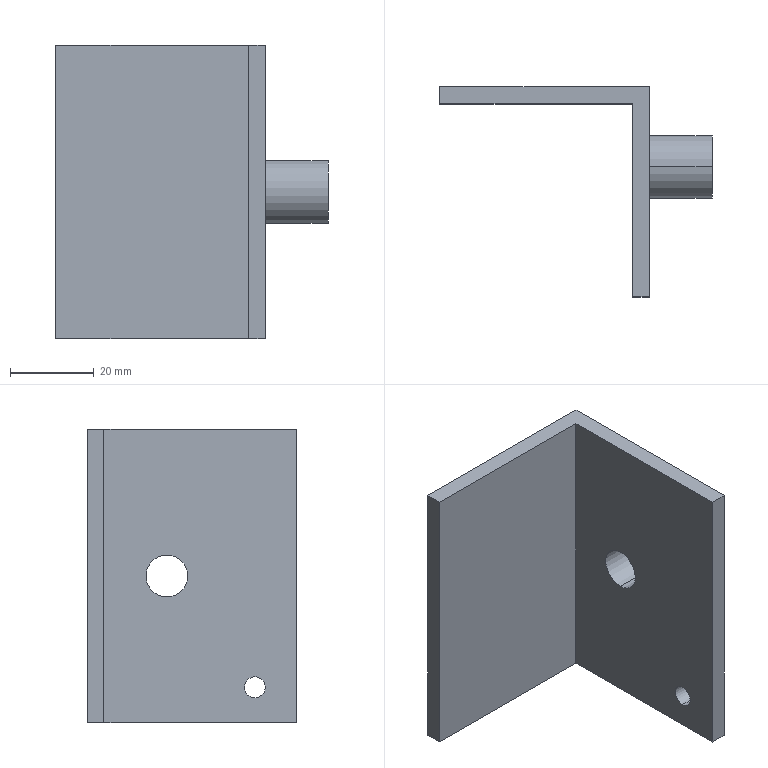Part | STEP file | 1 solid | 15 faces | box 65 x 50 x 70 mm | volume 27960 mm3 | plane 9 | cylinder 6 | commonest cylinder face diameters 5 x2 10 x2 15 x2
STEP:
#1=CARTESIAN_POINT('',(0.,0.,0.));
#2=DIRECTION('',(0.,0.,1.));
#3=DIRECTION('',(1.,0.,0.));
#4=AXIS2_PLACEMENT_3D('',#1,#2,#3);
#5=CARTESIAN_POINT('',(34.103,0.4017,42.5));
#6=VERTEX_POINT('',#5);
#7=CARTESIAN_POINT('',(34.103,0.4017,27.5));
#8=VERTEX_POINT('',#7);
#9=CARTESIAN_POINT('',(34.103,0.4017,35.));
#10=DIRECTION('',(-1.,0.,0.));
#11=DIRECTION('',(0.,0.,-1.));
#12=AXIS2_PLACEMENT_3D('',#9,#10,#11);
#13=CIRCLE('',#12,7.5);
#14=CARTESIAN_POINT('',(34.103,0.4017,35.));
#15=DIRECTION('',(1.,0.,0.));
#16=DIRECTION('',(0.,0.,-1.));
#17=AXIS2_PLACEMENT_3D('',#14,#15,#16);
#18=CYLINDRICAL_SURFACE('',#17,7.5);
#19=CARTESIAN_POINT('',(6.283,0.));
#20=DIRECTION('',(-1.,0.));
#21=VECTOR('',#20,1.);
#22=LINE('',#19,#21);
#23=(GEOMETRIC_REPRESENTATION_CONTEXT(2)PARAMETRIC_REPRESENTATION_CONTEXT()REPRESENTATION_CONTEXT('',''));
#24=DEFINITIONAL_REPRESENTATION('',(#22),#23);
#25=PCURVE('',#18,#24);
#26=CARTESIAN_POINT('',(34.103,-30.598,0.));
#27=DIRECTION('',(1.,0.,0.));
#28=DIRECTION('',(0.,0.,-1.));
#29=AXIS2_PLACEMENT_3D('',#26,#27,#28);
#30=PLANE('',#29);
#31=CARTESIAN_POINT('',(-27.5,31.));
#32=CARTESIAN_POINT('',(-27.5,18.01));
#33=CARTESIAN_POINT('',(-38.75,24.505));
#34=CARTESIAN_POINT('',(-50.,31.));
#35=CARTESIAN_POINT('',(-38.75,37.495));
#36=CARTESIAN_POINT('',(-27.5,43.99));
#37=CARTESIAN_POINT('',(-27.5,31.));
#38=(BOUNDED_CURVE()B_SPLINE_CURVE(2,(#31,#32,#33,#34,#35,#36,#37),.UNSPECIFIED.,.T.,.F.)B_SPLINE_CURVE_WITH_KNOTS((1,2,2,2,2,1),(-2.094,0.,2.094,4.189,6.283,8.378),.UNSPECIFIED.)CURVE()GEOMETRIC_REPRESENTATION_ITEM()RATIONAL_B_SPLINE_CURVE((1.,0.5,1.,0.5,1.,0.5,1.))REPRESENTATION_ITEM(''));
#39=(GEOMETRIC_REPRESENTATION_CONTEXT(2)PARAMETRIC_REPRESENTATION_CONTEXT()REPRESENTATION_CONTEXT('',''));
#40=DEFINITIONAL_REPRESENTATION('',(#38),#39);
#41=PCURVE('',#30,#40);
#42=SURFACE_CURVE('',#13,(#25,#41),.PCURVE_S1.);
#43=EDGE_CURVE('',#6,#8,#42,.T.);
#44=ORIENTED_EDGE('',*,*,#43,.F.);
#45=CARTESIAN_POINT('',(49.103,0.4017,42.5));
#46=VERTEX_POINT('',#45);
#47=CARTESIAN_POINT('',(34.103,0.4017,42.5));
#48=DIRECTION('',(1.,0.,0.));
#49=VECTOR('',#48,1.);
#50=LINE('',#47,#49);
#51=CARTESIAN_POINT('',(3.142,0.));
#52=DIRECTION('',(0.,1.));
#53=VECTOR('',#52,1.);
#54=LINE('',#51,#53);
#55=(GEOMETRIC_REPRESENTATION_CONTEXT(2)PARAMETRIC_REPRESENTATION_CONTEXT()REPRESENTATION_CONTEXT('',''));
#56=DEFINITIONAL_REPRESENTATION('',(#54),#55);
#57=PCURVE('',#18,#56);
#58=CARTESIAN_POINT('',(34.103,0.4017,35.));
#59=DIRECTION('',(1.,0.,0.));
#60=DIRECTION('',(0.,0.,-1.));
#61=AXIS2_PLACEMENT_3D('',#58,#59,#60);
#62=CYLINDRICAL_SURFACE('',#61,7.5);
#63=CARTESIAN_POINT('',(3.142,0.));
#64=DIRECTION('',(0.,1.));
#65=VECTOR('',#64,1.);
#66=LINE('',#63,#65);
#67=(GEOMETRIC_REPRESENTATION_CONTEXT(2)PARAMETRIC_REPRESENTATION_CONTEXT()REPRESENTATION_CONTEXT('',''));
#68=DEFINITIONAL_REPRESENTATION('',(#66),#67);
#69=PCURVE('',#62,#68);
#70=SURFACE_CURVE('',#50,(#57,#69),.PCURVE_S1.);
#71=EDGE_CURVE('',#6,#46,#70,.T.);
#72=ORIENTED_EDGE('',*,*,#71,.T.);
#73=CARTESIAN_POINT('',(49.103,0.4017,27.5));
#74=VERTEX_POINT('',#73);
#75=CARTESIAN_POINT('',(49.103,0.4017,35.));
#76=DIRECTION('',(-1.,0.,0.));
#77=DIRECTION('',(0.,0.,-1.));
#78=AXIS2_PLACEMENT_3D('',#75,#76,#77);
#79=CIRCLE('',#78,7.5);
#80=CARTESIAN_POINT('',(6.283,15.));
#81=DIRECTION('',(-1.,0.));
#82=VECTOR('',#81,1.);
#83=LINE('',#80,#82);
#84=(GEOMETRIC_REPRESENTATION_CONTEXT(2)PARAMETRIC_REPRESENTATION_CONTEXT()REPRESENTATION_CONTEXT('',''));
#85=DEFINITIONAL_REPRESENTATION('',(#83),#84);
#86=PCURVE('',#18,#85);
#87=CARTESIAN_POINT('',(49.103,0.4017,35.));
#88=DIRECTION('',(1.,0.,0.));
#89=DIRECTION('',(0.,0.,-1.));
#90=AXIS2_PLACEMENT_3D('',#87,#88,#89);
#91=PLANE('',#90);
#92=CARTESIAN_POINT('',(7.5,0.));
#93=CARTESIAN_POINT('',(7.5,-12.99));
#94=CARTESIAN_POINT('',(-3.75,-6.495));
#95=CARTESIAN_POINT('',(-15.,0.));
#96=CARTESIAN_POINT('',(-3.75,6.495));
#97=CARTESIAN_POINT('',(7.5,12.99));
#98=CARTESIAN_POINT('',(7.5,0.));
#99=(BOUNDED_CURVE()B_SPLINE_CURVE(2,(#92,#93,#94,#95,#96,#97,#98),.UNSPECIFIED.,.T.,.F.)B_SPLINE_CURVE_WITH_KNOTS((1,2,2,2,2,1),(-2.094,0.,2.094,4.189,6.283,8.378),.UNSPECIFIED.)CURVE()GEOMETRIC_REPRESENTATION_ITEM()RATIONAL_B_SPLINE_CURVE((1.,0.5,1.,0.5,1.,0.5,1.))REPRESENTATION_ITEM(''));
#100=(GEOMETRIC_REPRESENTATION_CONTEXT(2)PARAMETRIC_REPRESENTATION_CONTEXT()REPRESENTATION_CONTEXT('',''));
#101=DEFINITIONAL_REPRESENTATION('',(#99),#100);
#102=PCURVE('',#91,#101);
#103=SURFACE_CURVE('',#79,(#86,#102),.PCURVE_S1.);
#104=EDGE_CURVE('',#46,#74,#103,.T.);
#105=ORIENTED_EDGE('',*,*,#104,.T.);
#106=CARTESIAN_POINT('',(34.103,0.4017,27.5));
#107=DIRECTION('',(1.,0.,0.));
#108=VECTOR('',#107,1.);
#109=LINE('',#106,#108);
#110=CARTESIAN_POINT('',(0.,0.));
#111=DIRECTION('',(0.,1.));
#112=VECTOR('',#111,1.);
#113=LINE('',#110,#112);
#114=(GEOMETRIC_REPRESENTATION_CONTEXT(2)PARAMETRIC_REPRESENTATION_CONTEXT()REPRESENTATION_CONTEXT('',''));
#115=DEFINITIONAL_REPRESENTATION('',(#113),#114);
#116=PCURVE('',#18,#115);
#117=CARTESIAN_POINT('',(6.283,0.));
#118=DIRECTION('',(0.,1.));
#119=VECTOR('',#118,1.);
#120=LINE('',#117,#119);
#121=(GEOMETRIC_REPRESENTATION_CONTEXT(2)PARAMETRIC_REPRESENTATION_CONTEXT()REPRESENTATION_CONTEXT('',''));
#122=DEFINITIONAL_REPRESENTATION('',(#120),#121);
#123=PCURVE('',#62,#122);
#124=SURFACE_CURVE('',#109,(#116,#123),.PCURVE_S1.);
#125=EDGE_CURVE('',#8,#74,#124,.T.);
#126=ORIENTED_EDGE('',*,*,#125,.F.);
#127=EDGE_LOOP('',(#44,#72,#105,#126));
#128=FACE_BOUND('',#127,.T.);
#129=ADVANCED_FACE('',(#128),#18,.T.);
#130=CARTESIAN_POINT('',(34.103,-20.598,10.952));
#131=VERTEX_POINT('',#130);
#132=CARTESIAN_POINT('',(30.103,-20.598,10.952));
#133=VERTEX_POINT('',#132);
#134=CARTESIAN_POINT('',(34.103,-20.598,10.952));
#135=DIRECTION('',(-1.,0.,0.));
#136=VECTOR('',#135,1.);
#137=LINE('',#134,#136);
#138=CARTESIAN_POINT('',(34.103,-20.598,8.452));
#139=DIRECTION('',(-1.,0.,0.));
#140=DIRECTION('',(0.,0.,1.));
#141=AXIS2_PLACEMENT_3D('',#138,#139,#140);
#142=CYLINDRICAL_SURFACE('',#141,2.5);
#143=CARTESIAN_POINT('',(6.283,0.));
#144=DIRECTION('',(0.,1.));
#145=VECTOR('',#144,1.);
#146=LINE('',#143,#145);
#147=(GEOMETRIC_REPRESENTATION_CONTEXT(2)PARAMETRIC_REPRESENTATION_CONTEXT()REPRESENTATION_CONTEXT('',''));
#148=DEFINITIONAL_REPRESENTATION('',(#146),#147);
#149=PCURVE('',#142,#148);
#150=CARTESIAN_POINT('',(34.103,-20.598,8.452));
#151=DIRECTION('',(-1.,0.,0.));
#152=DIRECTION('',(0.,0.,1.));
#153=AXIS2_PLACEMENT_3D('',#150,#151,#152);
#154=CYLINDRICAL_SURFACE('',#153,2.5);
#155=CARTESIAN_POINT('',(0.,0.));
#156=DIRECTION('',(0.,1.));
#157=VECTOR('',#156,1.);
#158=LINE('',#155,#157);
#159=(GEOMETRIC_REPRESENTATION_CONTEXT(2)PARAMETRIC_REPRESENTATION_CONTEXT()REPRESENTATION_CONTEXT('',''));
#160=DEFINITIONAL_REPRESENTATION('',(#158),#159);
#161=PCURVE('',#154,#160);
#162=SURFACE_CURVE('',#137,(#149,#161),.PCURVE_S1.);
#163=EDGE_CURVE('',#131,#133,#162,.T.);
#164=ORIENTED_EDGE('',*,*,#163,.T.);
#165=CARTESIAN_POINT('',(30.103,-20.598,5.952));
#166=VERTEX_POINT('',#165);
#167=CARTESIAN_POINT('',(30.103,-20.598,8.452));
#168=DIRECTION('',(1.,0.,0.));
#169=DIRECTION('',(0.,0.,1.));
#170=AXIS2_PLACEMENT_3D('',#167,#168,#169);
#171=CIRCLE('',#170,2.5);
#172=CARTESIAN_POINT('',(6.283,4.));
#173=DIRECTION('',(-1.,0.));
#174=VECTOR('',#173,1.);
#175=LINE('',#172,#174);
#176=(GEOMETRIC_REPRESENTATION_CONTEXT(2)PARAMETRIC_REPRESENTATION_CONTEXT()REPRESENTATION_CONTEXT('',''));
#177=DEFINITIONAL_REPRESENTATION('',(#175),#176);
#178=PCURVE('',#142,#177);
#179=CARTESIAN_POINT('',(30.103,15.402,0.));
#180=DIRECTION('',(-1.,0.,0.));
#181=DIRECTION('',(0.,-1.,0.));
#182=AXIS2_PLACEMENT_3D('',#179,#180,#181);
#183=PLANE('',#182);
#184=CARTESIAN_POINT('',(36.,10.952));
#185=CARTESIAN_POINT('',(40.33,10.952));
#186=CARTESIAN_POINT('',(38.165,7.202));
#187=CARTESIAN_POINT('',(36.,3.452));
#188=CARTESIAN_POINT('',(33.835,7.202));
#189=CARTESIAN_POINT('',(31.67,10.952));
#190=CARTESIAN_POINT('',(36.,10.952));
#191=(BOUNDED_CURVE()B_SPLINE_CURVE(2,(#184,#185,#186,#187,#188,#189,#190),.UNSPECIFIED.,.T.,.F.)B_SPLINE_CURVE_WITH_KNOTS((1,2,2,2,2,1),(-2.094,0.,2.094,4.189,6.283,8.378),.UNSPECIFIED.)CURVE()GEOMETRIC_REPRESENTATION_ITEM()RATIONAL_B_SPLINE_CURVE((1.,0.5,1.,0.5,1.,0.5,1.))REPRESENTATION_ITEM(''));
#192=(GEOMETRIC_REPRESENTATION_CONTEXT(2)PARAMETRIC_REPRESENTATION_CONTEXT()REPRESENTATION_CONTEXT('',''));
#193=DEFINITIONAL_REPRESENTATION('',(#191),#192);
#194=PCURVE('',#183,#193);
#195=SURFACE_CURVE('',#171,(#178,#194),.PCURVE_S1.);
#196=EDGE_CURVE('',#133,#166,#195,.T.);
#197=ORIENTED_EDGE('',*,*,#196,.T.);
#198=CARTESIAN_POINT('',(34.103,-20.598,5.952));
#199=VERTEX_POINT('',#198);
#200=CARTESIAN_POINT('',(34.103,-20.598,5.952));
#201=DIRECTION('',(-1.,0.,0.));
#202=VECTOR('',#201,1.);
#203=LINE('',#200,#202);
#204=CARTESIAN_POINT('',(3.142,0.));
#205=DIRECTION('',(0.,1.));
#206=VECTOR('',#205,1.);
#207=LINE('',#204,#206);
#208=(GEOMETRIC_REPRESENTATION_CONTEXT(2)PARAMETRIC_REPRESENTATION_CONTEXT()REPRESENTATION_CONTEXT('',''));
#209=DEFINITIONAL_REPRESENTATION('',(#207),#208);
#210=PCURVE('',#142,#209);
#211=CARTESIAN_POINT('',(3.142,0.));
#212=DIRECTION('',(0.,1.));
#213=VECTOR('',#212,1.);
#214=LINE('',#211,#213);
#215=(GEOMETRIC_REPRESENTATION_CONTEXT(2)PARAMETRIC_REPRESENTATION_CONTEXT()REPRESENTATION_CONTEXT('',''));
#216=DEFINITIONAL_REPRESENTATION('',(#214),#215);
#217=PCURVE('',#154,#216);
#218=SURFACE_CURVE('',#203,(#210,#217),.PCURVE_S1.);
#219=EDGE_CURVE('',#199,#166,#218,.T.);
#220=ORIENTED_EDGE('',*,*,#219,.F.);
#221=CARTESIAN_POINT('',(34.103,-20.598,8.452));
#222=DIRECTION('',(-1.,0.,0.));
#223=DIRECTION('',(0.,0.,1.));
#224=AXIS2_PLACEMENT_3D('',#221,#222,#223);
#225=CIRCLE('',#224,2.5);
#226=CARTESIAN_POINT('',(0.,0.));
#227=DIRECTION('',(1.,0.));
#228=VECTOR('',#227,1.);
#229=LINE('',#226,#228);
#230=(GEOMETRIC_REPRESENTATION_CONTEXT(2)PARAMETRIC_REPRESENTATION_CONTEXT()REPRESENTATION_CONTEXT('',''));
#231=DEFINITIONAL_REPRESENTATION('',(#229),#230);
#232=PCURVE('',#142,#231);
#233=CARTESIAN_POINT('',(-10.952,10.));
#234=CARTESIAN_POINT('',(-10.952,14.33));
#235=CARTESIAN_POINT('',(-7.202,12.165));
#236=CARTESIAN_POINT('',(-3.452,10.));
#237=CARTESIAN_POINT('',(-7.202,7.835));
#238=CARTESIAN_POINT('',(-10.952,5.67));
#239=CARTESIAN_POINT('',(-10.952,10.));
#240=(BOUNDED_CURVE()B_SPLINE_CURVE(2,(#233,#234,#235,#236,#237,#238,#239),.UNSPECIFIED.,.T.,.F.)B_SPLINE_CURVE_WITH_KNOTS((1,2,2,2,2,1),(-2.094,0.,2.094,4.189,6.283,8.378),.UNSPECIFIED.)CURVE()GEOMETRIC_REPRESENTATION_ITEM()RATIONAL_B_SPLINE_CURVE((1.,0.5,1.,0.5,1.,0.5,1.))REPRESENTATION_ITEM(''));
#241=(GEOMETRIC_REPRESENTATION_CONTEXT(2)PARAMETRIC_REPRESENTATION_CONTEXT()REPRESENTATION_CONTEXT('',''));
#242=DEFINITIONAL_REPRESENTATION('',(#240),#241);
#243=PCURVE('',#30,#242);
#244=SURFACE_CURVE('',#225,(#232,#243),.PCURVE_S1.);
#245=EDGE_CURVE('',#199,#131,#244,.T.);
#246=ORIENTED_EDGE('',*,*,#245,.T.);
#247=EDGE_LOOP('',(#164,#197,#220,#246));
#248=FACE_BOUND('',#247,.F.);
#249=ADVANCED_FACE('',(#248),#142,.F.);
#250=CARTESIAN_POINT('',(30.103,0.4017,30.));
#251=VERTEX_POINT('',#250);
#252=CARTESIAN_POINT('',(49.103,0.4017,30.));
#253=VERTEX_POINT('',#252);
#254=CARTESIAN_POINT('',(34.103,0.4017,30.));
#255=DIRECTION('',(1.,0.,0.));
#256=VECTOR('',#255,1.);
#257=LINE('',#254,#256);
#258=CARTESIAN_POINT('',(34.103,0.4017,35.));
#259=DIRECTION('',(1.,0.,0.));
#260=DIRECTION('',(0.,0.,-1.));
#261=AXIS2_PLACEMENT_3D('',#258,#259,#260);
#262=CYLINDRICAL_SURFACE('',#261,5.);
#263=CARTESIAN_POINT('',(6.283,0.));
#264=DIRECTION('',(0.,1.));
#265=VECTOR('',#264,1.);
#266=LINE('',#263,#265);
#267=(GEOMETRIC_REPRESENTATION_CONTEXT(2)PARAMETRIC_REPRESENTATION_CONTEXT()REPRESENTATION_CONTEXT('',''));
#268=DEFINITIONAL_REPRESENTATION('',(#266),#267);
#269=PCURVE('',#262,#268);
#270=CARTESIAN_POINT('',(34.103,0.4017,35.));
#271=DIRECTION('',(1.,0.,0.));
#272=DIRECTION('',(0.,0.,-1.));
#273=AXIS2_PLACEMENT_3D('',#270,#271,#272);
#274=CYLINDRICAL_SURFACE('',#273,5.);
#275=CARTESIAN_POINT('',(0.,0.));
#276=DIRECTION('',(0.,1.));
#277=VECTOR('',#276,1.);
#278=LINE('',#275,#277);
#279=(GEOMETRIC_REPRESENTATION_CONTEXT(2)PARAMETRIC_REPRESENTATION_CONTEXT()REPRESENTATION_CONTEXT('',''));
#280=DEFINITIONAL_REPRESENTATION('',(#278),#279);
#281=PCURVE('',#274,#280);
#282=SURFACE_CURVE('',#257,(#269,#281),.PCURVE_S1.);
#283=EDGE_CURVE('',#251,#253,#282,.T.);
#284=ORIENTED_EDGE('',*,*,#283,.T.);
#285=CARTESIAN_POINT('',(49.103,0.4017,40.));
#286=VERTEX_POINT('',#285);
#287=CARTESIAN_POINT('',(49.103,0.4017,35.));
#288=DIRECTION('',(-1.,0.,0.));
#289=DIRECTION('',(0.,0.,-1.));
#290=AXIS2_PLACEMENT_3D('',#287,#288,#289);
#291=CIRCLE('',#290,5.);
#292=CARTESIAN_POINT('',(6.283,15.));
#293=DIRECTION('',(-1.,0.));
#294=VECTOR('',#293,1.);
#295=LINE('',#292,#294);
#296=(GEOMETRIC_REPRESENTATION_CONTEXT(2)PARAMETRIC_REPRESENTATION_CONTEXT()REPRESENTATION_CONTEXT('',''));
#297=DEFINITIONAL_REPRESENTATION('',(#295),#296);
#298=PCURVE('',#262,#297);
#299=CARTESIAN_POINT('',(5.,0.));
#300=CARTESIAN_POINT('',(5.,-8.66));
#301=CARTESIAN_POINT('',(-2.5,-4.33));
#302=CARTESIAN_POINT('',(-10.,0.));
#303=CARTESIAN_POINT('',(-2.5,4.33));
#304=CARTESIAN_POINT('',(5.,8.66));
#305=CARTESIAN_POINT('',(5.,0.));
#306=(BOUNDED_CURVE()B_SPLINE_CURVE(2,(#299,#300,#301,#302,#303,#304,#305),.UNSPECIFIED.,.T.,.F.)B_SPLINE_CURVE_WITH_KNOTS((1,2,2,2,2,1),(-2.094,0.,2.094,4.189,6.283,8.378),.UNSPECIFIED.)CURVE()GEOMETRIC_REPRESENTATION_ITEM()RATIONAL_B_SPLINE_CURVE((1.,0.5,1.,0.5,1.,0.5,1.))REPRESENTATION_ITEM(''));
#307=(GEOMETRIC_REPRESENTATION_CONTEXT(2)PARAMETRIC_REPRESENTATION_CONTEXT()REPRESENTATION_CONTEXT('',''));
#308=DEFINITIONAL_REPRESENTATION('',(#306),#307);
#309=PCURVE('',#91,#308);
#310=SURFACE_CURVE('',#291,(#298,#309),.PCURVE_S1.);
#311=EDGE_CURVE('',#253,#286,#310,.T.);
#312=ORIENTED_EDGE('',*,*,#311,.T.);
#313=CARTESIAN_POINT('',(30.103,0.4017,40.));
#314=VERTEX_POINT('',#313);
#315=CARTESIAN_POINT('',(34.103,0.4017,40.));
#316=DIRECTION('',(1.,0.,0.));
#317=VECTOR('',#316,1.);
#318=LINE('',#315,#317);
#319=CARTESIAN_POINT('',(3.142,0.));
#320=DIRECTION('',(0.,1.));
#321=VECTOR('',#320,1.);
#322=LINE('',#319,#321);
#323=(GEOMETRIC_REPRESENTATION_CONTEXT(2)PARAMETRIC_REPRESENTATION_CONTEXT()REPRESENTATION_CONTEXT('',''));
#324=DEFINITIONAL_REPRESENTATION('',(#322),#323);
#325=PCURVE('',#262,#324);
#326=CARTESIAN_POINT('',(3.142,0.));
#327=DIRECTION('',(0.,1.));
#328=VECTOR('',#327,1.);
#329=LINE('',#326,#328);
#330=(GEOMETRIC_REPRESENTATION_CONTEXT(2)PARAMETRIC_REPRESENTATION_CONTEXT()REPRESENTATION_CONTEXT('',''));
#331=DEFINITIONAL_REPRESENTATION('',(#329),#330);
#332=PCURVE('',#274,#331);
#333=SURFACE_CURVE('',#318,(#325,#332),.PCURVE_S1.);
#334=EDGE_CURVE('',#314,#286,#333,.T.);
#335=ORIENTED_EDGE('',*,*,#334,.F.);
#336=CARTESIAN_POINT('',(30.103,0.4017,35.));
#337=DIRECTION('',(1.,0.,0.));
#338=DIRECTION('',(0.,0.,-1.));
#339=AXIS2_PLACEMENT_3D('',#336,#337,#338);
#340=CIRCLE('',#339,5.);
#341=CARTESIAN_POINT('',(0.,-4.));
#342=DIRECTION('',(1.,0.));
#343=VECTOR('',#342,1.);
#344=LINE('',#341,#343);
#345=(GEOMETRIC_REPRESENTATION_CONTEXT(2)PARAMETRIC_REPRESENTATION_CONTEXT()REPRESENTATION_CONTEXT('',''));
#346=DEFINITIONAL_REPRESENTATION('',(#344),#345);
#347=PCURVE('',#262,#346);
#348=CARTESIAN_POINT('',(15.,30.));
#349=CARTESIAN_POINT('',(6.34,30.));
#350=CARTESIAN_POINT('',(10.67,37.5));
#351=CARTESIAN_POINT('',(15.,45.));
#352=CARTESIAN_POINT('',(19.33,37.5));
#353=CARTESIAN_POINT('',(23.66,30.));
#354=CARTESIAN_POINT('',(15.,30.));
#355=(BOUNDED_CURVE()B_SPLINE_CURVE(2,(#348,#349,#350,#351,#352,#353,#354),.UNSPECIFIED.,.T.,.F.)B_SPLINE_CURVE_WITH_KNOTS((1,2,2,2,2,1),(-2.094,0.,2.094,4.189,6.283,8.378),.UNSPECIFIED.)CURVE()GEOMETRIC_REPRESENTATION_ITEM()RATIONAL_B_SPLINE_CURVE((1.,0.5,1.,0.5,1.,0.5,1.))REPRESENTATION_ITEM(''));
#356=(GEOMETRIC_REPRESENTATION_CONTEXT(2)PARAMETRIC_REPRESENTATION_CONTEXT()REPRESENTATION_CONTEXT('',''));
#357=DEFINITIONAL_REPRESENTATION('',(#355),#356);
#358=PCURVE('',#183,#357);
#359=SURFACE_CURVE('',#340,(#347,#358),.PCURVE_S1.);
#360=EDGE_CURVE('',#314,#251,#359,.T.);
#361=ORIENTED_EDGE('',*,*,#360,.T.);
#362=EDGE_LOOP('',(#284,#312,#335,#361));
#363=FACE_BOUND('',#362,.F.);
#364=ADVANCED_FACE('',(#363),#262,.F.);
#365=CARTESIAN_POINT('',(-15.897,19.402,70.));
#366=VERTEX_POINT('',#365);
#367=CARTESIAN_POINT('',(34.103,19.402,70.));
#368=VERTEX_POINT('',#367);
#369=CARTESIAN_POINT('',(34.103,19.402,70.));
#370=DIRECTION('',(1.,0.,0.));
#371=VECTOR('',#370,1.);
#372=LINE('',#369,#371);
#373=CARTESIAN_POINT('',(34.103,19.402,0.));
#374=DIRECTION('',(0.,1.,0.));
#375=DIRECTION('',(0.,0.,1.));
#376=AXIS2_PLACEMENT_3D('',#373,#374,#375);
#377=PLANE('',#376);
#378=CARTESIAN_POINT('',(70.,0.));
#379=DIRECTION('',(0.,1.));
#380=VECTOR('',#379,1.);
#381=LINE('',#378,#380);
#382=(GEOMETRIC_REPRESENTATION_CONTEXT(2)PARAMETRIC_REPRESENTATION_CONTEXT()REPRESENTATION_CONTEXT('',''));
#383=DEFINITIONAL_REPRESENTATION('',(#381),#382);
#384=PCURVE('',#377,#383);
#385=CARTESIAN_POINT('',(19.683,4.982,70.));
#386=DIRECTION('',(0.,0.,1.));
#387=DIRECTION('',(1.,0.,0.));
#388=AXIS2_PLACEMENT_3D('',#385,#386,#387);
#389=PLANE('',#388);
#390=CARTESIAN_POINT('',(14.42,14.42));
#391=DIRECTION('',(1.,0.));
#392=VECTOR('',#391,1.);
#393=LINE('',#390,#392);
#394=(GEOMETRIC_REPRESENTATION_CONTEXT(2)PARAMETRIC_REPRESENTATION_CONTEXT()REPRESENTATION_CONTEXT('',''));
#395=DEFINITIONAL_REPRESENTATION('',(#393),#394);
#396=PCURVE('',#389,#395);
#397=SURFACE_CURVE('',#372,(#384,#396),.PCURVE_S1.);
#398=EDGE_CURVE('',#366,#368,#397,.T.);
#399=ORIENTED_EDGE('',*,*,#398,.T.);
#400=CARTESIAN_POINT('',(34.103,19.402,0.));
#401=VERTEX_POINT('',#400);
#402=CARTESIAN_POINT('',(34.103,19.402,0.));
#403=DIRECTION('',(0.,0.,-1.));
#404=VECTOR('',#403,1.);
#405=LINE('',#402,#404);
#406=CARTESIAN_POINT('',(0.,0.));
#407=DIRECTION('',(-1.,0.));
#408=VECTOR('',#407,1.);
#409=LINE('',#406,#408);
#410=(GEOMETRIC_REPRESENTATION_CONTEXT(2)PARAMETRIC_REPRESENTATION_CONTEXT()REPRESENTATION_CONTEXT('',''));
#411=DEFINITIONAL_REPRESENTATION('',(#409),#410);
#412=PCURVE('',#377,#411);
#413=CARTESIAN_POINT('',(0.,50.));
#414=DIRECTION('',(1.,0.));
#415=VECTOR('',#414,1.);
#416=LINE('',#413,#415);
#417=(GEOMETRIC_REPRESENTATION_CONTEXT(2)PARAMETRIC_REPRESENTATION_CONTEXT()REPRESENTATION_CONTEXT('',''));
#418=DEFINITIONAL_REPRESENTATION('',(#416),#417);
#419=PCURVE('',#30,#418);
#420=SURFACE_CURVE('',#405,(#412,#419),.PCURVE_S1.);
#421=EDGE_CURVE('',#368,#401,#420,.T.);
#422=ORIENTED_EDGE('',*,*,#421,.T.);
#423=CARTESIAN_POINT('',(-15.897,19.402,0.));
#424=VERTEX_POINT('',#423);
#425=CARTESIAN_POINT('',(34.103,19.402,0.));
#426=DIRECTION('',(-1.,0.,0.));
#427=VECTOR('',#426,1.);
#428=LINE('',#425,#427);
#429=CARTESIAN_POINT('',(0.,0.));
#430=DIRECTION('',(0.,-1.));
#431=VECTOR('',#430,1.);
#432=LINE('',#429,#431);
#433=(GEOMETRIC_REPRESENTATION_CONTEXT(2)PARAMETRIC_REPRESENTATION_CONTEXT()REPRESENTATION_CONTEXT('',''));
#434=DEFINITIONAL_REPRESENTATION('',(#432),#433);
#435=PCURVE('',#377,#434);
#436=CARTESIAN_POINT('',(19.683,4.982,0.));
#437=DIRECTION('',(0.,0.,1.));
#438=DIRECTION('',(1.,0.,0.));
#439=AXIS2_PLACEMENT_3D('',#436,#437,#438);
#440=PLANE('',#439);
#441=CARTESIAN_POINT('',(14.42,14.42));
#442=DIRECTION('',(-1.,0.));
#443=VECTOR('',#442,1.);
#444=LINE('',#441,#443);
#445=(GEOMETRIC_REPRESENTATION_CONTEXT(2)PARAMETRIC_REPRESENTATION_CONTEXT()REPRESENTATION_CONTEXT('',''));
#446=DEFINITIONAL_REPRESENTATION('',(#444),#445);
#447=PCURVE('',#440,#446);
#448=SURFACE_CURVE('',#428,(#435,#447),.PCURVE_S1.);
#449=EDGE_CURVE('',#401,#424,#448,.T.);
#450=ORIENTED_EDGE('',*,*,#449,.T.);
#451=CARTESIAN_POINT('',(-15.897,19.402,0.));
#452=DIRECTION('',(0.,0.,1.));
#453=VECTOR('',#452,1.);
#454=LINE('',#451,#453);
#455=CARTESIAN_POINT('',(0.,-50.));
#456=DIRECTION('',(1.,0.));
#457=VECTOR('',#456,1.);
#458=LINE('',#455,#457);
#459=(GEOMETRIC_REPRESENTATION_CONTEXT(2)PARAMETRIC_REPRESENTATION_CONTEXT()REPRESENTATION_CONTEXT('',''));
#460=DEFINITIONAL_REPRESENTATION('',(#458),#459);
#461=PCURVE('',#377,#460);
#462=CARTESIAN_POINT('',(-15.897,19.402,0.));
#463=DIRECTION('',(-1.,0.,0.));
#464=DIRECTION('',(0.,-1.,0.));
#465=AXIS2_PLACEMENT_3D('',#462,#463,#464);
#466=PLANE('',#465);
#467=CARTESIAN_POINT('',(0.,0.));
#468=DIRECTION('',(0.,1.));
#469=VECTOR('',#468,1.);
#470=LINE('',#467,#469);
#471=(GEOMETRIC_REPRESENTATION_CONTEXT(2)PARAMETRIC_REPRESENTATION_CONTEXT()REPRESENTATION_CONTEXT('',''));
#472=DEFINITIONAL_REPRESENTATION('',(#470),#471);
#473=PCURVE('',#466,#472);
#474=SURFACE_CURVE('',#454,(#461,#473),.PCURVE_S1.);
#475=EDGE_CURVE('',#424,#366,#474,.T.);
#476=ORIENTED_EDGE('',*,*,#475,.T.);
#477=EDGE_LOOP('',(#399,#422,#450,#476));
#478=FACE_BOUND('',#477,.T.);
#479=ADVANCED_FACE('',(#478),#377,.T.);
#480=CARTESIAN_POINT('',(34.103,0.4017,35.));
#481=DIRECTION('',(-1.,0.,0.));
#482=DIRECTION('',(0.,0.,-1.));
#483=AXIS2_PLACEMENT_3D('',#480,#481,#482);
#484=CIRCLE('',#483,7.5);
#485=CARTESIAN_POINT('',(-27.5,31.));
#486=CARTESIAN_POINT('',(-27.5,18.01));
#487=CARTESIAN_POINT('',(-38.75,24.505));
#488=CARTESIAN_POINT('',(-50.,31.));
#489=CARTESIAN_POINT('',(-38.75,37.495));
#490=CARTESIAN_POINT('',(-27.5,43.99));
#491=CARTESIAN_POINT('',(-27.5,31.));
#492=(BOUNDED_CURVE()B_SPLINE_CURVE(2,(#485,#486,#487,#488,#489,#490,#491),.UNSPECIFIED.,.T.,.F.)B_SPLINE_CURVE_WITH_KNOTS((1,2,2,2,2,1),(-2.094,0.,2.094,4.189,6.283,8.378),.UNSPECIFIED.)CURVE()GEOMETRIC_REPRESENTATION_ITEM()RATIONAL_B_SPLINE_CURVE((1.,0.5,1.,0.5,1.,0.5,1.))REPRESENTATION_ITEM(''));
#493=(GEOMETRIC_REPRESENTATION_CONTEXT(2)PARAMETRIC_REPRESENTATION_CONTEXT()REPRESENTATION_CONTEXT('',''));
#494=DEFINITIONAL_REPRESENTATION('',(#492),#493);
#495=PCURVE('',#30,#494);
#496=CARTESIAN_POINT('',(6.283,0.));
#497=DIRECTION('',(-1.,0.));
#498=VECTOR('',#497,1.);
#499=LINE('',#496,#498);
#500=(GEOMETRIC_REPRESENTATION_CONTEXT(2)PARAMETRIC_REPRESENTATION_CONTEXT()REPRESENTATION_CONTEXT('',''));
#501=DEFINITIONAL_REPRESENTATION('',(#499),#500);
#502=PCURVE('',#62,#501);
#503=SURFACE_CURVE('',#484,(#495,#502),.PCURVE_S1.);
#504=EDGE_CURVE('',#8,#6,#503,.T.);
#505=ORIENTED_EDGE('',*,*,#504,.T.);
#506=ORIENTED_EDGE('',*,*,#43,.T.);
#507=EDGE_LOOP('',(#505,#506));
#508=FACE_BOUND('',#507,.T.);
#509=CARTESIAN_POINT('',(34.103,-20.598,8.452));
#510=DIRECTION('',(-1.,0.,0.));
#511=DIRECTION('',(0.,0.,1.));
#512=AXIS2_PLACEMENT_3D('',#509,#510,#511);
#513=CIRCLE('',#512,2.5);
#514=CARTESIAN_POINT('',(-10.952,10.));
#515=CARTESIAN_POINT('',(-10.952,14.33));
#516=CARTESIAN_POINT('',(-7.202,12.165));
#517=CARTESIAN_POINT('',(-3.452,10.));
#518=CARTESIAN_POINT('',(-7.202,7.835));
#519=CARTESIAN_POINT('',(-10.952,5.67));
#520=CARTESIAN_POINT('',(-10.952,10.));
#521=(BOUNDED_CURVE()B_SPLINE_CURVE(2,(#514,#515,#516,#517,#518,#519,#520),.UNSPECIFIED.,.T.,.F.)B_SPLINE_CURVE_WITH_KNOTS((1,2,2,2,2,1),(-2.094,0.,2.094,4.189,6.283,8.378),.UNSPECIFIED.)CURVE()GEOMETRIC_REPRESENTATION_ITEM()RATIONAL_B_SPLINE_CURVE((1.,0.5,1.,0.5,1.,0.5,1.))REPRESENTATION_ITEM(''));
#522=(GEOMETRIC_REPRESENTATION_CONTEXT(2)PARAMETRIC_REPRESENTATION_CONTEXT()REPRESENTATION_CONTEXT('',''));
#523=DEFINITIONAL_REPRESENTATION('',(#521),#522);
#524=PCURVE('',#30,#523);
#525=CARTESIAN_POINT('',(0.,0.));
#526=DIRECTION('',(1.,0.));
#527=VECTOR('',#526,1.);
#528=LINE('',#525,#527);
#529=(GEOMETRIC_REPRESENTATION_CONTEXT(2)PARAMETRIC_REPRESENTATION_CONTEXT()REPRESENTATION_CONTEXT('',''));
#530=DEFINITIONAL_REPRESENTATION('',(#528),#529);
#531=PCURVE('',#154,#530);
#532=SURFACE_CURVE('',#513,(#524,#531),.PCURVE_S1.);
#533=EDGE_CURVE('',#131,#199,#532,.T.);
#534=ORIENTED_EDGE('',*,*,#533,.T.);
#535=ORIENTED_EDGE('',*,*,#245,.T.);
#536=EDGE_LOOP('',(#534,#535));
#537=FACE_BOUND('',#536,.T.);
#538=CARTESIAN_POINT('',(34.103,-30.598,70.));
#539=VERTEX_POINT('',#538);
#540=CARTESIAN_POINT('',(34.103,-30.598,70.));
#541=DIRECTION('',(0.,-1.,0.));
#542=VECTOR('',#541,1.);
#543=LINE('',#540,#542);
#544=CARTESIAN_POINT('',(-70.,0.));
#545=DIRECTION('',(0.,-1.));
#546=VECTOR('',#545,1.);
#547=LINE('',#544,#546);
#548=(GEOMETRIC_REPRESENTATION_CONTEXT(2)PARAMETRIC_REPRESENTATION_CONTEXT()REPRESENTATION_CONTEXT('',''));
#549=DEFINITIONAL_REPRESENTATION('',(#547),#548);
#550=PCURVE('',#30,#549);
#551=CARTESIAN_POINT('',(14.42,-35.58));
#552=DIRECTION('',(0.,-1.));
#553=VECTOR('',#552,1.);
#554=LINE('',#551,#553);
#555=(GEOMETRIC_REPRESENTATION_CONTEXT(2)PARAMETRIC_REPRESENTATION_CONTEXT()REPRESENTATION_CONTEXT('',''));
#556=DEFINITIONAL_REPRESENTATION('',(#554),#555);
#557=PCURVE('',#389,#556);
#558=SURFACE_CURVE('',#543,(#550,#557),.PCURVE_S1.);
#559=EDGE_CURVE('',#368,#539,#558,.T.);
#560=ORIENTED_EDGE('',*,*,#559,.T.);
#561=CARTESIAN_POINT('',(34.103,-30.598,0.));
#562=VERTEX_POINT('',#561);
#563=CARTESIAN_POINT('',(34.103,-30.598,0.));
#564=DIRECTION('',(0.,0.,-1.));
#565=VECTOR('',#564,1.);
#566=LINE('',#563,#565);
#567=CARTESIAN_POINT('',(0.,0.));
#568=DIRECTION('',(1.,0.));
#569=VECTOR('',#568,1.);
#570=LINE('',#567,#569);
#571=(GEOMETRIC_REPRESENTATION_CONTEXT(2)PARAMETRIC_REPRESENTATION_CONTEXT()REPRESENTATION_CONTEXT('',''));
#572=DEFINITIONAL_REPRESENTATION('',(#570),#571);
#573=PCURVE('',#30,#572);
#574=CARTESIAN_POINT('',(30.103,-30.598,0.));
#575=DIRECTION('',(0.,-1.,0.));
#576=DIRECTION('',(0.,0.,-1.));
#577=AXIS2_PLACEMENT_3D('',#574,#575,#576);
#578=PLANE('',#577);
#579=CARTESIAN_POINT('',(0.,4.));
#580=DIRECTION('',(1.,0.));
#581=VECTOR('',#580,1.);
#582=LINE('',#579,#581);
#583=(GEOMETRIC_REPRESENTATION_CONTEXT(2)PARAMETRIC_REPRESENTATION_CONTEXT()REPRESENTATION_CONTEXT('',''));
#584=DEFINITIONAL_REPRESENTATION('',(#582),#583);
#585=PCURVE('',#578,#584);
#586=SURFACE_CURVE('',#566,(#573,#585),.PCURVE_S1.);
#587=EDGE_CURVE('',#539,#562,#586,.T.);
#588=ORIENTED_EDGE('',*,*,#587,.T.);
#589=CARTESIAN_POINT('',(34.103,-30.598,0.));
#590=DIRECTION('',(0.,1.,0.));
#591=VECTOR('',#590,1.);
#592=LINE('',#589,#591);
#593=CARTESIAN_POINT('',(0.,0.));
#594=DIRECTION('',(0.,1.));
#595=VECTOR('',#594,1.);
#596=LINE('',#593,#595);
#597=(GEOMETRIC_REPRESENTATION_CONTEXT(2)PARAMETRIC_REPRESENTATION_CONTEXT()REPRESENTATION_CONTEXT('',''));
#598=DEFINITIONAL_REPRESENTATION('',(#596),#597);
#599=PCURVE('',#30,#598);
#600=CARTESIAN_POINT('',(14.42,-35.58));
#601=DIRECTION('',(0.,1.));
#602=VECTOR('',#601,1.);
#603=LINE('',#600,#602);
#604=(GEOMETRIC_REPRESENTATION_CONTEXT(2)PARAMETRIC_REPRESENTATION_CONTEXT()REPRESENTATION_CONTEXT('',''));
#605=DEFINITIONAL_REPRESENTATION('',(#603),#604);
#606=PCURVE('',#440,#605);
#607=SURFACE_CURVE('',#592,(#599,#606),.PCURVE_S1.);
#608=EDGE_CURVE('',#562,#401,#607,.T.);
#609=ORIENTED_EDGE('',*,*,#608,.T.);
#610=ORIENTED_EDGE('',*,*,#421,.F.);
#611=EDGE_LOOP('',(#560,#588,#609,#610));
#612=FACE_BOUND('',#611,.T.);
#613=ADVANCED_FACE('',(#508,#537,#612),#30,.T.);
#614=CARTESIAN_POINT('',(30.103,-30.598,70.));
#615=VERTEX_POINT('',#614);
#616=CARTESIAN_POINT('',(19.683,-30.598,70.));
#617=DIRECTION('',(1.,0.,0.));
#618=VECTOR('',#617,1.);
#619=LINE('',#616,#618);
#620=CARTESIAN_POINT('',(0.,-35.58));
#621=DIRECTION('',(1.,0.));
#622=VECTOR('',#621,1.);
#623=LINE('',#620,#622);
#624=(GEOMETRIC_REPRESENTATION_CONTEXT(2)PARAMETRIC_REPRESENTATION_CONTEXT()REPRESENTATION_CONTEXT('',''));
#625=DEFINITIONAL_REPRESENTATION('',(#623),#624);
#626=PCURVE('',#389,#625);
#627=CARTESIAN_POINT('',(-70.,-10.42));
#628=DIRECTION('',(0.,1.));
#629=VECTOR('',#628,1.);
#630=LINE('',#627,#629);
#631=(GEOMETRIC_REPRESENTATION_CONTEXT(2)PARAMETRIC_REPRESENTATION_CONTEXT()REPRESENTATION_CONTEXT('',''));
#632=DEFINITIONAL_REPRESENTATION('',(#630),#631);
#633=PCURVE('',#578,#632);
#634=SURFACE_CURVE('',#619,(#626,#633),.PCURVE_S1.);
#635=EDGE_CURVE('',#615,#539,#634,.T.);
#636=ORIENTED_EDGE('',*,*,#635,.T.);
#637=ORIENTED_EDGE('',*,*,#559,.F.);
#638=ORIENTED_EDGE('',*,*,#398,.F.);
#639=CARTESIAN_POINT('',(-15.897,15.402,70.));
#640=VERTEX_POINT('',#639);
#641=CARTESIAN_POINT('',(-15.897,4.982,70.));
#642=DIRECTION('',(0.,-1.,0.));
#643=VECTOR('',#642,1.);
#644=LINE('',#641,#643);
#645=CARTESIAN_POINT('',(-35.58,0.));
#646=DIRECTION('',(0.,-1.));
#647=VECTOR('',#646,1.);
#648=LINE('',#645,#647);
#649=(GEOMETRIC_REPRESENTATION_CONTEXT(2)PARAMETRIC_REPRESENTATION_CONTEXT()REPRESENTATION_CONTEXT('',''));
#650=DEFINITIONAL_REPRESENTATION('',(#648),#649);
#651=PCURVE('',#389,#650);
#652=CARTESIAN_POINT('',(14.42,70.));
#653=DIRECTION('',(1.,0.));
#654=VECTOR('',#653,1.);
#655=LINE('',#652,#654);
#656=(GEOMETRIC_REPRESENTATION_CONTEXT(2)PARAMETRIC_REPRESENTATION_CONTEXT()REPRESENTATION_CONTEXT('',''));
#657=DEFINITIONAL_REPRESENTATION('',(#655),#656);
#658=PCURVE('',#466,#657);
#659=SURFACE_CURVE('',#644,(#651,#658),.PCURVE_S1.);
#660=EDGE_CURVE('',#366,#640,#659,.T.);
#661=ORIENTED_EDGE('',*,*,#660,.T.);
#662=CARTESIAN_POINT('',(30.103,15.402,70.));
#663=VERTEX_POINT('',#662);
#664=CARTESIAN_POINT('',(19.683,15.402,70.));
#665=DIRECTION('',(1.,0.,0.));
#666=VECTOR('',#665,1.);
#667=LINE('',#664,#666);
#668=CARTESIAN_POINT('',(0.,10.42));
#669=DIRECTION('',(1.,0.));
#670=VECTOR('',#669,1.);
#671=LINE('',#668,#670);
#672=(GEOMETRIC_REPRESENTATION_CONTEXT(2)PARAMETRIC_REPRESENTATION_CONTEXT()REPRESENTATION_CONTEXT('',''));
#673=DEFINITIONAL_REPRESENTATION('',(#671),#672);
#674=PCURVE('',#389,#673);
#675=CARTESIAN_POINT('',(-15.897,15.402,0.));
#676=DIRECTION('',(0.,-1.,0.));
#677=DIRECTION('',(1.,0.,0.));
#678=AXIS2_PLACEMENT_3D('',#675,#676,#677);
#679=PLANE('',#678);
#680=CARTESIAN_POINT('',(35.58,70.));
#681=DIRECTION('',(1.,0.));
#682=VECTOR('',#681,1.);
#683=LINE('',#680,#682);
#684=(GEOMETRIC_REPRESENTATION_CONTEXT(2)PARAMETRIC_REPRESENTATION_CONTEXT()REPRESENTATION_CONTEXT('',''));
#685=DEFINITIONAL_REPRESENTATION('',(#683),#684);
#686=PCURVE('',#679,#685);
#687=SURFACE_CURVE('',#667,(#674,#686),.PCURVE_S1.);
#688=EDGE_CURVE('',#640,#663,#687,.T.);
#689=ORIENTED_EDGE('',*,*,#688,.T.);
#690=CARTESIAN_POINT('',(30.103,4.982,70.));
#691=DIRECTION('',(0.,-1.,0.));
#692=VECTOR('',#691,1.);
#693=LINE('',#690,#692);
#694=CARTESIAN_POINT('',(10.42,0.));
#695=DIRECTION('',(0.,-1.));
#696=VECTOR('',#695,1.);
#697=LINE('',#694,#696);
#698=(GEOMETRIC_REPRESENTATION_CONTEXT(2)PARAMETRIC_REPRESENTATION_CONTEXT()REPRESENTATION_CONTEXT('',''));
#699=DEFINITIONAL_REPRESENTATION('',(#697),#698);
#700=PCURVE('',#389,#699);
#701=CARTESIAN_POINT('',(10.42,70.));
#702=DIRECTION('',(1.,0.));
#703=VECTOR('',#702,1.);
#704=LINE('',#701,#703);
#705=(GEOMETRIC_REPRESENTATION_CONTEXT(2)PARAMETRIC_REPRESENTATION_CONTEXT()REPRESENTATION_CONTEXT('',''));
#706=DEFINITIONAL_REPRESENTATION('',(#704),#705);
#707=PCURVE('',#183,#706);
#708=SURFACE_CURVE('',#693,(#700,#707),.PCURVE_S1.);
#709=EDGE_CURVE('',#663,#615,#708,.T.);
#710=ORIENTED_EDGE('',*,*,#709,.T.);
#711=EDGE_LOOP('',(#636,#637,#638,#661,#689,#710));
#712=FACE_BOUND('',#711,.T.);
#713=ADVANCED_FACE('',(#712),#389,.T.);
#714=ORIENTED_EDGE('',*,*,#660,.F.);
#715=ORIENTED_EDGE('',*,*,#475,.F.);
#716=CARTESIAN_POINT('',(-15.897,15.402,0.));
#717=VERTEX_POINT('',#716);
#718=CARTESIAN_POINT('',(-15.897,19.402,0.));
#719=DIRECTION('',(0.,-1.,0.));
#720=VECTOR('',#719,1.);
#721=LINE('',#718,#720);
#722=CARTESIAN_POINT('',(0.,0.));
#723=DIRECTION('',(1.,0.));
#724=VECTOR('',#723,1.);
#725=LINE('',#722,#724);
#726=(GEOMETRIC_REPRESENTATION_CONTEXT(2)PARAMETRIC_REPRESENTATION_CONTEXT()REPRESENTATION_CONTEXT('',''));
#727=DEFINITIONAL_REPRESENTATION('',(#725),#726);
#728=PCURVE('',#466,#727);
#729=CARTESIAN_POINT('',(-35.58,14.42));
#730=DIRECTION('',(0.,-1.));
#731=VECTOR('',#730,1.);
#732=LINE('',#729,#731);
#733=(GEOMETRIC_REPRESENTATION_CONTEXT(2)PARAMETRIC_REPRESENTATION_CONTEXT()REPRESENTATION_CONTEXT('',''));
#734=DEFINITIONAL_REPRESENTATION('',(#732),#733);
#735=PCURVE('',#440,#734);
#736=SURFACE_CURVE('',#721,(#728,#735),.PCURVE_S1.);
#737=EDGE_CURVE('',#424,#717,#736,.T.);
#738=ORIENTED_EDGE('',*,*,#737,.T.);
#739=CARTESIAN_POINT('',(-15.897,15.402,0.));
#740=DIRECTION('',(0.,0.,1.));
#741=VECTOR('',#740,1.);
#742=LINE('',#739,#741);
#743=CARTESIAN_POINT('',(4.,0.));
#744=DIRECTION('',(0.,1.));
#745=VECTOR('',#744,1.);
#746=LINE('',#743,#745);
#747=(GEOMETRIC_REPRESENTATION_CONTEXT(2)PARAMETRIC_REPRESENTATION_CONTEXT()REPRESENTATION_CONTEXT('',''));
#748=DEFINITIONAL_REPRESENTATION('',(#746),#747);
#749=PCURVE('',#466,#748);
#750=CARTESIAN_POINT('',(0.,0.));
#751=DIRECTION('',(0.,1.));
#752=VECTOR('',#751,1.);
#753=LINE('',#750,#752);
#754=(GEOMETRIC_REPRESENTATION_CONTEXT(2)PARAMETRIC_REPRESENTATION_CONTEXT()REPRESENTATION_CONTEXT('',''));
#755=DEFINITIONAL_REPRESENTATION('',(#753),#754);
#756=PCURVE('',#679,#755);
#757=SURFACE_CURVE('',#742,(#749,#756),.PCURVE_S1.);
#758=EDGE_CURVE('',#717,#640,#757,.T.);
#759=ORIENTED_EDGE('',*,*,#758,.T.);
#760=EDGE_LOOP('',(#714,#715,#738,#759));
#761=FACE_BOUND('',#760,.T.);
#762=ADVANCED_FACE('',(#761),#466,.T.);
#763=ORIENTED_EDGE('',*,*,#608,.F.);
#764=CARTESIAN_POINT('',(30.103,-30.598,0.));
#765=VERTEX_POINT('',#764);
#766=CARTESIAN_POINT('',(19.683,-30.598,0.));
#767=DIRECTION('',(1.,0.,0.));
#768=VECTOR('',#767,1.);
#769=LINE('',#766,#768);
#770=CARTESIAN_POINT('',(0.,-35.58));
#771=DIRECTION('',(1.,0.));
#772=VECTOR('',#771,1.);
#773=LINE('',#770,#772);
#774=(GEOMETRIC_REPRESENTATION_CONTEXT(2)PARAMETRIC_REPRESENTATION_CONTEXT()REPRESENTATION_CONTEXT('',''));
#775=DEFINITIONAL_REPRESENTATION('',(#773),#774);
#776=PCURVE('',#440,#775);
#777=CARTESIAN_POINT('',(0.,-10.42));
#778=DIRECTION('',(0.,1.));
#779=VECTOR('',#778,1.);
#780=LINE('',#777,#779);
#781=(GEOMETRIC_REPRESENTATION_CONTEXT(2)PARAMETRIC_REPRESENTATION_CONTEXT()REPRESENTATION_CONTEXT('',''));
#782=DEFINITIONAL_REPRESENTATION('',(#780),#781);
#783=PCURVE('',#578,#782);
#784=SURFACE_CURVE('',#769,(#776,#783),.PCURVE_S1.);
#785=EDGE_CURVE('',#765,#562,#784,.T.);
#786=ORIENTED_EDGE('',*,*,#785,.F.);
#787=CARTESIAN_POINT('',(30.103,15.402,0.));
#788=VERTEX_POINT('',#787);
#789=CARTESIAN_POINT('',(30.103,4.982,0.));
#790=DIRECTION('',(0.,-1.,0.));
#791=VECTOR('',#790,1.);
#792=LINE('',#789,#791);
#793=CARTESIAN_POINT('',(10.42,0.));
#794=DIRECTION('',(0.,-1.));
#795=VECTOR('',#794,1.);
#796=LINE('',#793,#795);
#797=(GEOMETRIC_REPRESENTATION_CONTEXT(2)PARAMETRIC_REPRESENTATION_CONTEXT()REPRESENTATION_CONTEXT('',''));
#798=DEFINITIONAL_REPRESENTATION('',(#796),#797);
#799=PCURVE('',#440,#798);
#800=CARTESIAN_POINT('',(10.42,0.));
#801=DIRECTION('',(1.,0.));
#802=VECTOR('',#801,1.);
#803=LINE('',#800,#802);
#804=(GEOMETRIC_REPRESENTATION_CONTEXT(2)PARAMETRIC_REPRESENTATION_CONTEXT()REPRESENTATION_CONTEXT('',''));
#805=DEFINITIONAL_REPRESENTATION('',(#803),#804);
#806=PCURVE('',#183,#805);
#807=SURFACE_CURVE('',#792,(#799,#806),.PCURVE_S1.);
#808=EDGE_CURVE('',#788,#765,#807,.T.);
#809=ORIENTED_EDGE('',*,*,#808,.F.);
#810=CARTESIAN_POINT('',(19.683,15.402,0.));
#811=DIRECTION('',(1.,0.,0.));
#812=VECTOR('',#811,1.);
#813=LINE('',#810,#812);
#814=CARTESIAN_POINT('',(0.,10.42));
#815=DIRECTION('',(1.,0.));
#816=VECTOR('',#815,1.);
#817=LINE('',#814,#816);
#818=(GEOMETRIC_REPRESENTATION_CONTEXT(2)PARAMETRIC_REPRESENTATION_CONTEXT()REPRESENTATION_CONTEXT('',''));
#819=DEFINITIONAL_REPRESENTATION('',(#817),#818);
#820=PCURVE('',#440,#819);
#821=CARTESIAN_POINT('',(35.58,0.));
#822=DIRECTION('',(1.,0.));
#823=VECTOR('',#822,1.);
#824=LINE('',#821,#823);
#825=(GEOMETRIC_REPRESENTATION_CONTEXT(2)PARAMETRIC_REPRESENTATION_CONTEXT()REPRESENTATION_CONTEXT('',''));
#826=DEFINITIONAL_REPRESENTATION('',(#824),#825);
#827=PCURVE('',#679,#826);
#828=SURFACE_CURVE('',#813,(#820,#827),.PCURVE_S1.);
#829=EDGE_CURVE('',#717,#788,#828,.T.);
#830=ORIENTED_EDGE('',*,*,#829,.F.);
#831=ORIENTED_EDGE('',*,*,#737,.F.);
#832=ORIENTED_EDGE('',*,*,#449,.F.);
#833=EDGE_LOOP('',(#763,#786,#809,#830,#831,#832));
#834=FACE_BOUND('',#833,.T.);
#835=ADVANCED_FACE('',(#834),#440,.F.);
#836=ORIENTED_EDGE('',*,*,#71,.F.);
#837=ORIENTED_EDGE('',*,*,#504,.F.);
#838=ORIENTED_EDGE('',*,*,#125,.T.);
#839=CARTESIAN_POINT('',(49.103,0.4017,35.));
#840=DIRECTION('',(-1.,0.,0.));
#841=DIRECTION('',(0.,0.,-1.));
#842=AXIS2_PLACEMENT_3D('',#839,#840,#841);
#843=CIRCLE('',#842,7.5);
#844=CARTESIAN_POINT('',(6.283,15.));
#845=DIRECTION('',(-1.,0.));
#846=VECTOR('',#845,1.);
#847=LINE('',#844,#846);
#848=(GEOMETRIC_REPRESENTATION_CONTEXT(2)PARAMETRIC_REPRESENTATION_CONTEXT()REPRESENTATION_CONTEXT('',''));
#849=DEFINITIONAL_REPRESENTATION('',(#847),#848);
#850=PCURVE('',#62,#849);
#851=CARTESIAN_POINT('',(7.5,0.));
#852=CARTESIAN_POINT('',(7.5,-12.99));
#853=CARTESIAN_POINT('',(-3.75,-6.495));
#854=CARTESIAN_POINT('',(-15.,0.));
#855=CARTESIAN_POINT('',(-3.75,6.495));
#856=CARTESIAN_POINT('',(7.5,12.99));
#857=CARTESIAN_POINT('',(7.5,0.));
#858=(BOUNDED_CURVE()B_SPLINE_CURVE(2,(#851,#852,#853,#854,#855,#856,#857),.UNSPECIFIED.,.T.,.F.)B_SPLINE_CURVE_WITH_KNOTS((1,2,2,2,2,1),(-2.094,0.,2.094,4.189,6.283,8.378),.UNSPECIFIED.)CURVE()GEOMETRIC_REPRESENTATION_ITEM()RATIONAL_B_SPLINE_CURVE((1.,0.5,1.,0.5,1.,0.5,1.))REPRESENTATION_ITEM(''));
#859=(GEOMETRIC_REPRESENTATION_CONTEXT(2)PARAMETRIC_REPRESENTATION_CONTEXT()REPRESENTATION_CONTEXT('',''));
#860=DEFINITIONAL_REPRESENTATION('',(#858),#859);
#861=PCURVE('',#91,#860);
#862=SURFACE_CURVE('',#843,(#850,#861),.PCURVE_S1.);
#863=EDGE_CURVE('',#74,#46,#862,.T.);
#864=ORIENTED_EDGE('',*,*,#863,.T.);
#865=EDGE_LOOP('',(#836,#837,#838,#864));
#866=FACE_BOUND('',#865,.T.);
#867=ADVANCED_FACE('',(#866),#62,.T.);
#868=CARTESIAN_POINT('',(30.103,-20.598,8.452));
#869=DIRECTION('',(1.,0.,0.));
#870=DIRECTION('',(0.,0.,1.));
#871=AXIS2_PLACEMENT_3D('',#868,#869,#870);
#872=CIRCLE('',#871,2.5);
#873=CARTESIAN_POINT('',(6.283,4.));
#874=DIRECTION('',(-1.,0.));
#875=VECTOR('',#874,1.);
#876=LINE('',#873,#875);
#877=(GEOMETRIC_REPRESENTATION_CONTEXT(2)PARAMETRIC_REPRESENTATION_CONTEXT()REPRESENTATION_CONTEXT('',''));
#878=DEFINITIONAL_REPRESENTATION('',(#876),#877);
#879=PCURVE('',#154,#878);
#880=CARTESIAN_POINT('',(36.,10.952));
#881=CARTESIAN_POINT('',(40.33,10.952));
#882=CARTESIAN_POINT('',(38.165,7.202));
#883=CARTESIAN_POINT('',(36.,3.452));
#884=CARTESIAN_POINT('',(33.835,7.202));
#885=CARTESIAN_POINT('',(31.67,10.952));
#886=CARTESIAN_POINT('',(36.,10.952));
#887=(BOUNDED_CURVE()B_SPLINE_CURVE(2,(#880,#881,#882,#883,#884,#885,#886),.UNSPECIFIED.,.T.,.F.)B_SPLINE_CURVE_WITH_KNOTS((1,2,2,2,2,1),(-2.094,0.,2.094,4.189,6.283,8.378),.UNSPECIFIED.)CURVE()GEOMETRIC_REPRESENTATION_ITEM()RATIONAL_B_SPLINE_CURVE((1.,0.5,1.,0.5,1.,0.5,1.))REPRESENTATION_ITEM(''));
#888=(GEOMETRIC_REPRESENTATION_CONTEXT(2)PARAMETRIC_REPRESENTATION_CONTEXT()REPRESENTATION_CONTEXT('',''));
#889=DEFINITIONAL_REPRESENTATION('',(#887),#888);
#890=PCURVE('',#183,#889);
#891=SURFACE_CURVE('',#872,(#879,#890),.PCURVE_S1.);
#892=EDGE_CURVE('',#166,#133,#891,.T.);
#893=ORIENTED_EDGE('',*,*,#892,.T.);
#894=ORIENTED_EDGE('',*,*,#163,.F.);
#895=ORIENTED_EDGE('',*,*,#533,.T.);
#896=ORIENTED_EDGE('',*,*,#219,.T.);
#897=EDGE_LOOP('',(#893,#894,#895,#896));
#898=FACE_BOUND('',#897,.F.);
#899=ADVANCED_FACE('',(#898),#154,.F.);
#900=ORIENTED_EDGE('',*,*,#635,.F.);
#901=CARTESIAN_POINT('',(30.103,-30.598,0.));
#902=DIRECTION('',(0.,0.,-1.));
#903=VECTOR('',#902,1.);
#904=LINE('',#901,#903);
#905=CARTESIAN_POINT('',(0.,0.));
#906=DIRECTION('',(1.,0.));
#907=VECTOR('',#906,1.);
#908=LINE('',#905,#907);
#909=(GEOMETRIC_REPRESENTATION_CONTEXT(2)PARAMETRIC_REPRESENTATION_CONTEXT()REPRESENTATION_CONTEXT('',''));
#910=DEFINITIONAL_REPRESENTATION('',(#908),#909);
#911=PCURVE('',#578,#910);
#912=CARTESIAN_POINT('',(46.,0.));
#913=DIRECTION('',(0.,-1.));
#914=VECTOR('',#913,1.);
#915=LINE('',#912,#914);
#916=(GEOMETRIC_REPRESENTATION_CONTEXT(2)PARAMETRIC_REPRESENTATION_CONTEXT()REPRESENTATION_CONTEXT('',''));
#917=DEFINITIONAL_REPRESENTATION('',(#915),#916);
#918=PCURVE('',#183,#917);
#919=SURFACE_CURVE('',#904,(#911,#918),.PCURVE_S1.);
#920=EDGE_CURVE('',#615,#765,#919,.T.);
#921=ORIENTED_EDGE('',*,*,#920,.T.);
#922=ORIENTED_EDGE('',*,*,#785,.T.);
#923=ORIENTED_EDGE('',*,*,#587,.F.);
#924=EDGE_LOOP('',(#900,#921,#922,#923));
#925=FACE_BOUND('',#924,.T.);
#926=ADVANCED_FACE('',(#925),#578,.T.);
#927=ORIENTED_EDGE('',*,*,#709,.F.);
#928=CARTESIAN_POINT('',(30.103,15.402,0.));
#929=DIRECTION('',(0.,0.,-1.));
#930=VECTOR('',#929,1.);
#931=LINE('',#928,#930);
#932=CARTESIAN_POINT('',(0.,0.));
#933=DIRECTION('',(0.,-1.));
#934=VECTOR('',#933,1.);
#935=LINE('',#932,#934);
#936=(GEOMETRIC_REPRESENTATION_CONTEXT(2)PARAMETRIC_REPRESENTATION_CONTEXT()REPRESENTATION_CONTEXT('',''));
#937=DEFINITIONAL_REPRESENTATION('',(#935),#936);
#938=PCURVE('',#183,#937);
#939=CARTESIAN_POINT('',(46.,0.));
#940=DIRECTION('',(0.,-1.));
#941=VECTOR('',#940,1.);
#942=LINE('',#939,#941);
#943=(GEOMETRIC_REPRESENTATION_CONTEXT(2)PARAMETRIC_REPRESENTATION_CONTEXT()REPRESENTATION_CONTEXT('',''));
#944=DEFINITIONAL_REPRESENTATION('',(#942),#943);
#945=PCURVE('',#679,#944);
#946=SURFACE_CURVE('',#931,(#938,#945),.PCURVE_S1.);
#947=EDGE_CURVE('',#663,#788,#946,.T.);
#948=ORIENTED_EDGE('',*,*,#947,.T.);
#949=ORIENTED_EDGE('',*,*,#808,.T.);
#950=ORIENTED_EDGE('',*,*,#920,.F.);
#951=EDGE_LOOP('',(#927,#948,#949,#950));
#952=FACE_BOUND('',#951,.T.);
#953=ORIENTED_EDGE('',*,*,#196,.T.);
#954=ORIENTED_EDGE('',*,*,#892,.T.);
#955=EDGE_LOOP('',(#953,#954));
#956=FACE_BOUND('',#955,.T.);
#957=CARTESIAN_POINT('',(30.103,0.4017,35.));
#958=DIRECTION('',(1.,0.,0.));
#959=DIRECTION('',(0.,0.,-1.));
#960=AXIS2_PLACEMENT_3D('',#957,#958,#959);
#961=CIRCLE('',#960,5.);
#962=CARTESIAN_POINT('',(15.,30.));
#963=CARTESIAN_POINT('',(6.34,30.));
#964=CARTESIAN_POINT('',(10.67,37.5));
#965=CARTESIAN_POINT('',(15.,45.));
#966=CARTESIAN_POINT('',(19.33,37.5));
#967=CARTESIAN_POINT('',(23.66,30.));
#968=CARTESIAN_POINT('',(15.,30.));
#969=(BOUNDED_CURVE()B_SPLINE_CURVE(2,(#962,#963,#964,#965,#966,#967,#968),.UNSPECIFIED.,.T.,.F.)B_SPLINE_CURVE_WITH_KNOTS((1,2,2,2,2,1),(-2.094,0.,2.094,4.189,6.283,8.378),.UNSPECIFIED.)CURVE()GEOMETRIC_REPRESENTATION_ITEM()RATIONAL_B_SPLINE_CURVE((1.,0.5,1.,0.5,1.,0.5,1.))REPRESENTATION_ITEM(''));
#970=(GEOMETRIC_REPRESENTATION_CONTEXT(2)PARAMETRIC_REPRESENTATION_CONTEXT()REPRESENTATION_CONTEXT('',''));
#971=DEFINITIONAL_REPRESENTATION('',(#969),#970);
#972=PCURVE('',#183,#971);
#973=CARTESIAN_POINT('',(0.,-4.));
#974=DIRECTION('',(1.,0.));
#975=VECTOR('',#974,1.);
#976=LINE('',#973,#975);
#977=(GEOMETRIC_REPRESENTATION_CONTEXT(2)PARAMETRIC_REPRESENTATION_CONTEXT()REPRESENTATION_CONTEXT('',''));
#978=DEFINITIONAL_REPRESENTATION('',(#976),#977);
#979=PCURVE('',#274,#978);
#980=SURFACE_CURVE('',#961,(#972,#979),.PCURVE_S1.);
#981=EDGE_CURVE('',#251,#314,#980,.T.);
#982=ORIENTED_EDGE('',*,*,#981,.T.);
#983=ORIENTED_EDGE('',*,*,#360,.T.);
#984=EDGE_LOOP('',(#982,#983));
#985=FACE_BOUND('',#984,.T.);
#986=ADVANCED_FACE('',(#952,#956,#985),#183,.T.);
#987=ORIENTED_EDGE('',*,*,#688,.F.);
#988=ORIENTED_EDGE('',*,*,#758,.F.);
#989=ORIENTED_EDGE('',*,*,#829,.T.);
#990=ORIENTED_EDGE('',*,*,#947,.F.);
#991=EDGE_LOOP('',(#987,#988,#989,#990));
#992=FACE_BOUND('',#991,.T.);
#993=ADVANCED_FACE('',(#992),#679,.T.);
#994=ORIENTED_EDGE('',*,*,#863,.F.);
#995=ORIENTED_EDGE('',*,*,#104,.F.);
#996=EDGE_LOOP('',(#994,#995));
#997=FACE_BOUND('',#996,.T.);
#998=ORIENTED_EDGE('',*,*,#311,.T.);
#999=CARTESIAN_POINT('',(49.103,0.4017,35.));
#1000=DIRECTION('',(-1.,0.,0.));
#1001=DIRECTION('',(0.,0.,-1.));
#1002=AXIS2_PLACEMENT_3D('',#999,#1000,#1001);
#1003=CIRCLE('',#1002,5.);
#1004=CARTESIAN_POINT('',(5.,0.));
#1005=CARTESIAN_POINT('',(5.,-8.66));
#1006=CARTESIAN_POINT('',(-2.5,-4.33));
#1007=CARTESIAN_POINT('',(-10.,0.));
#1008=CARTESIAN_POINT('',(-2.5,4.33));
#1009=CARTESIAN_POINT('',(5.,8.66));
#1010=CARTESIAN_POINT('',(5.,0.));
#1011=(BOUNDED_CURVE()B_SPLINE_CURVE(2,(#1004,#1005,#1006,#1007,#1008,#1009,#1010),.UNSPECIFIED.,.T.,.F.)B_SPLINE_CURVE_WITH_KNOTS((1,2,2,2,2,1),(-2.094,0.,2.094,4.189,6.283,8.378),.UNSPECIFIED.)CURVE()GEOMETRIC_REPRESENTATION_ITEM()RATIONAL_B_SPLINE_CURVE((1.,0.5,1.,0.5,1.,0.5,1.))REPRESENTATION_ITEM(''));
#1012=(GEOMETRIC_REPRESENTATION_CONTEXT(2)PARAMETRIC_REPRESENTATION_CONTEXT()REPRESENTATION_CONTEXT('',''));
#1013=DEFINITIONAL_REPRESENTATION('',(#1011),#1012);
#1014=PCURVE('',#91,#1013);
#1015=CARTESIAN_POINT('',(6.283,15.));
#1016=DIRECTION('',(-1.,0.));
#1017=VECTOR('',#1016,1.);
#1018=LINE('',#1015,#1017);
#1019=(GEOMETRIC_REPRESENTATION_CONTEXT(2)PARAMETRIC_REPRESENTATION_CONTEXT()REPRESENTATION_CONTEXT('',''));
#1020=DEFINITIONAL_REPRESENTATION('',(#1018),#1019);
#1021=PCURVE('',#274,#1020);
#1022=SURFACE_CURVE('',#1003,(#1014,#1021),.PCURVE_S1.);
#1023=EDGE_CURVE('',#286,#253,#1022,.T.);
#1024=ORIENTED_EDGE('',*,*,#1023,.T.);
#1025=EDGE_LOOP('',(#998,#1024));
#1026=FACE_BOUND('',#1025,.T.);
#1027=ADVANCED_FACE('',(#997,#1026),#91,.T.);
#1028=ORIENTED_EDGE('',*,*,#1023,.T.);
#1029=ORIENTED_EDGE('',*,*,#283,.F.);
#1030=ORIENTED_EDGE('',*,*,#981,.T.);
#1031=ORIENTED_EDGE('',*,*,#334,.T.);
#1032=EDGE_LOOP('',(#1028,#1029,#1030,#1031));
#1033=FACE_BOUND('',#1032,.F.);
#1034=ADVANCED_FACE('',(#1033),#274,.F.);
#1035=CLOSED_SHELL('',(#129,#249,#364,#479,#613,#713,#762,#835,#867,#899,#926,#986,#993,#1027,#1034));
#1036=MANIFOLD_SOLID_BREP('',#1035);
#1037=(LENGTH_UNIT()NAMED_UNIT(*)SI_UNIT(.MILLI.,.METRE.));
#1038=UNCERTAINTY_MEASURE_WITH_UNIT(LENGTH_MEASURE(0.0000001),#1037,'','');
#1039=(NAMED_UNIT(*)PLANE_ANGLE_UNIT()SI_UNIT($,.RADIAN.));
#1040=(NAMED_UNIT(*)SI_UNIT($,.STERADIAN.)SOLID_ANGLE_UNIT());
#1041=(GEOMETRIC_REPRESENTATION_CONTEXT(3)GLOBAL_UNCERTAINTY_ASSIGNED_CONTEXT((#1038))GLOBAL_UNIT_ASSIGNED_CONTEXT((#1037,#1039,#1040))REPRESENTATION_CONTEXT('',''));
#1042=ADVANCED_BREP_SHAPE_REPRESENTATION('',(#4,#1036),#1041);